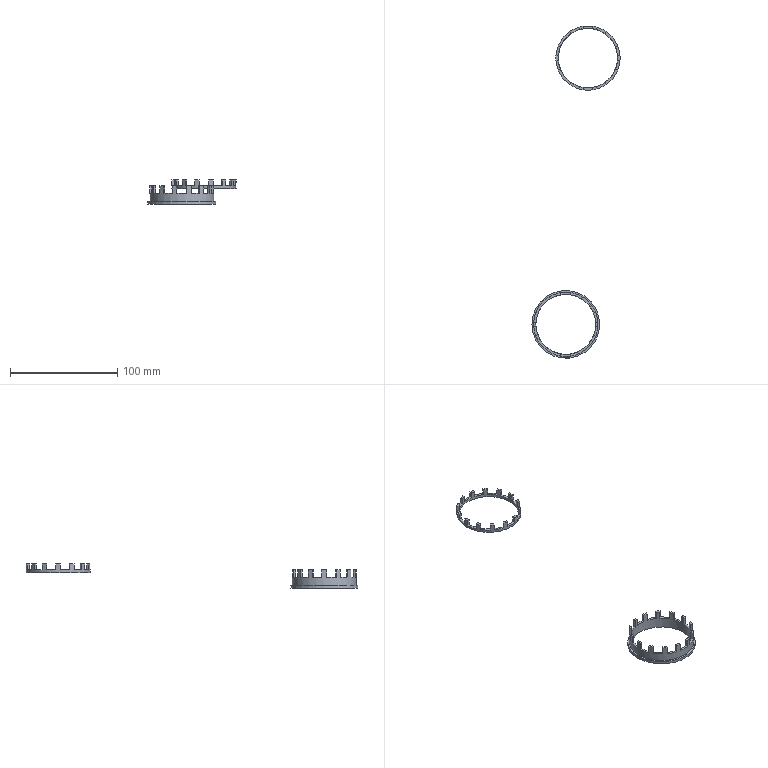NC program | NX | posted with a generic post | part box 82.344 x 310.506 x 22.5 mm
Lines 1 to 1001 of 7127:
N10 G17 G21 G94 G90
(ZLEVEL_PROFILE_COPY_13 , TOOL : D6)
N12 T06 M6
N14 G54
N16 G17 G0 G90 X-0.851 Y-23.489 S9500 M3
N18 G43 Z38. H6
N20 Z7.711
N22 G41 G94 G1 X-0.945 Y-23.523 F1000. D6
N24 X-1.203 Y-23.672
N26 G3 X-1.503 Y-24.192 R0.6
N28 G1 X-1.5 Y-27.4 F2200.
N30 Y-29.387
N32 Y-32.959
N34 G3 X-1.2 Y-33.479 R0.6
N36 G1 X-0.961 Y-33.617
N38 G40
N40 X-0.867 Y-33.651
N42 X0.891 Y-33.745
N44 G41 X0.984 Y-33.707 F1000.
N46 X1.226 Y-33.555
N48 G3 X1.506 Y-33.024 R0.6
N50 G1 X1.5 Y-32.851 F2200.
N52 Y-29.387
N54 Y-27.383
N56 X1.52 Y-27.041
N58 X1.5 Y-27.028
N60 X1.503 Y-24.192
N62 G3 X1.204 Y-23.672 R0.6
N64 G1 X0.945 Y-23.523
N66 G40
N68 X0.851 Y-23.488
N70 G0 X-0.851 Y-23.489 Z7.421
N72 G41 G1 X-0.945 Y-23.523 F1000.
N74 X-1.203 Y-23.672
N76 G3 X-1.503 Y-24.192 R0.6
N78 G1 X-1.5 Y-27.4 F2200.
N80 Y-29.387
N82 Y-32.959
N84 G3 X-1.2 Y-33.479 R0.6
N86 G1 X-0.961 Y-33.617
N88 G40
N90 X-0.867 Y-33.651
N92 X0.891 Y-33.745
N94 G41 X0.984 Y-33.707 F1000.
N96 X1.226 Y-33.555
N98 G3 X1.506 Y-33.024 R0.6
N100 G1 X1.5 Y-32.851 F2200.
N102 Y-29.387
N104 Y-27.383
N106 X1.52 Y-27.041
N108 X1.5 Y-27.028
N110 X1.503 Y-24.192
N112 G3 X1.204 Y-23.672 R0.6
N114 G1 X0.945 Y-23.523
N116 G40
N118 X0.851 Y-23.488
N120 G0 X-0.85 Y-23.489 Z7.132
N122 G41 G1 X-0.944 Y-23.523 F1000.
N124 X-1.203 Y-23.673
N126 G3 X-1.503 Y-24.192 R0.6
N128 G1 X-1.5 Y-27.4 F2200.
N130 Y-29.387
N132 Y-32.959
N134 G3 X-1.2 Y-33.479 R0.6
N136 G1 X-0.961 Y-33.617
N138 G40
N140 X-0.867 Y-33.651
N142 X0.891 Y-33.745
N144 G41 X0.984 Y-33.707 F1000.
N146 X1.226 Y-33.555
N148 G3 X1.506 Y-33.024 R0.6
N150 G1 X1.5 Y-32.851 F2200.
N152 Y-29.387
N154 Y-27.383
N156 X1.52 Y-27.041
N158 X1.5 Y-27.028
N160 X1.503 Y-24.192
N162 G3 X1.204 Y-23.672 R0.6
N164 G1 X0.945 Y-23.523
N166 G40
N168 X0.851 Y-23.488
N170 G0 X-0.85 Y-23.489 Z6.842
N172 G41 G1 X-0.944 Y-23.523 F1000.
N174 X-1.203 Y-23.673
N176 G3 X-1.503 Y-24.192 R0.6
N178 G1 X-1.5 Y-27.4 F2200.
N180 Y-29.387
N182 Y-32.959
N184 G3 X-1.2 Y-33.479 R0.6
N186 G1 X-0.96 Y-33.617
N188 G40
N190 X-0.866 Y-33.651
N192 X0.891 Y-33.745
N194 G41 X0.984 Y-33.707 F1000.
N196 X1.226 Y-33.555
N198 G3 X1.506 Y-33.024 R0.6
N200 G1 X1.5 Y-32.851 F2200.
N202 Y-29.387
N204 Y-27.383
N206 X1.52 Y-27.041
N208 X1.5 Y-27.028
N210 X1.503 Y-24.192
N212 G3 X1.204 Y-23.672 R0.6
N214 G1 X0.945 Y-23.523
N216 G40
N218 X0.851 Y-23.488
N220 G0 X-0.85 Y-23.489 Z6.553
N222 G41 G1 X-0.944 Y-23.523 F1000.
N224 X-1.203 Y-23.673
N226 G3 X-1.502 Y-24.192 R0.6
N228 G1 X-1.5 Y-27.4 F2200.
N230 Y-29.387
N232 Y-32.959
N234 G3 X-1.199 Y-33.479 R0.6
N236 G1 X-0.96 Y-33.617
N238 G40
N240 X-0.866 Y-33.651
N242 X0.891 Y-33.745
N244 G41 X0.984 Y-33.707 F1000.
N246 X1.226 Y-33.555
N248 G3 X1.506 Y-33.024 R0.6
N250 G1 X1.5 Y-32.851 F2200.
N252 Y-29.387
N254 Y-27.383
N256 X1.52 Y-27.041
N258 X1.5 Y-27.028
N260 X1.503 Y-24.192
N262 G3 X1.204 Y-23.672 R0.6
N264 G1 X0.945 Y-23.523
N266 G40
N268 X0.851 Y-23.488
N270 G0 X-0.85 Y-23.489 Z6.263
N272 G41 G1 X-0.944 Y-23.523 F1000.
N274 X-1.203 Y-23.673
N276 G3 X-1.502 Y-24.192 R0.6
N278 G1 X-1.5 Y-27.4 F2200.
N280 Y-29.387
N282 X-1.499 Y-32.959
N284 G3 X-1.199 Y-33.479 R0.6
N286 G1 X-0.96 Y-33.617
N288 G40
N290 X-0.866 Y-33.651
N292 X0.891 Y-33.745
N294 G41 X0.984 Y-33.707 F1000.
N296 X1.226 Y-33.555
N298 G3 X1.506 Y-33.024 R0.6
N300 G1 X1.499 Y-32.851 F2200.
N302 X1.5 Y-29.387
N304 X1.499 Y-27.383
N306 X1.52 Y-27.041
N308 X1.499 Y-27.028
N310 X1.503 Y-24.192
N312 G3 X1.204 Y-23.672 R0.6
N314 G1 X0.945 Y-23.523
N316 G40
N318 X0.851 Y-23.488
N320 G0 X-0.85 Y-23.489 Z5.974
N322 G41 G1 X-0.944 Y-23.523 F1000.
N324 X-1.203 Y-23.673
N326 G3 X-1.502 Y-24.192 R0.6
N328 G1 X-1.5 Y-27.4 F2200.
N330 Y-29.387
N332 X-1.499 Y-32.959
N334 G3 X-1.199 Y-33.479 R0.6
N336 G1 X-0.96 Y-33.617
N338 G40
N340 X-0.866 Y-33.651
N342 X0.891 Y-33.745
N344 G41 X0.984 Y-33.707 F1000.
N346 X1.226 Y-33.555
N348 G3 X1.506 Y-33.024 R0.6
N350 G1 X1.499 Y-32.851 F2200.
N352 X1.5 Y-29.387
N354 X1.499 Y-27.383
N356 X1.52 Y-27.041
N358 X1.499 Y-27.028
N360 X1.503 Y-24.192
N362 G3 X1.204 Y-23.672 R0.6
N364 G1 X0.945 Y-23.523
N366 G40
N368 X0.851 Y-23.488
N370 G0 X-0.85 Y-23.489 Z5.684
N372 G41 G1 X-0.944 Y-23.523 F1000.
N374 X-1.203 Y-23.673
N376 G3 X-1.502 Y-24.192 R0.6
N378 G1 X-1.5 Y-27.4 F2200.
N380 Y-29.387
N382 X-1.499 Y-32.959
N384 G3 X-1.199 Y-33.479 R0.6
N386 G1 X-0.96 Y-33.617
N388 G40
N390 X-0.866 Y-33.651
N392 X0.891 Y-33.745
N394 G41 X0.983 Y-33.707 F1000.
N396 X1.226 Y-33.555
N398 G3 X1.506 Y-33.024 R0.6
N400 G1 X1.499 Y-32.851 F2200.
N402 X1.5 Y-29.387
N404 X1.499 Y-27.383
N406 X1.52 Y-27.041
N408 X1.499 Y-27.028
N410 X1.503 Y-24.192
N412 G3 X1.204 Y-23.672 R0.6
N414 G1 X0.945 Y-23.523
N416 G40
N418 X0.851 Y-23.488
N420 G0 X-0.85 Y-23.489 Z5.395
N422 G41 G1 X-0.944 Y-23.523 F1000.
N424 X-1.202 Y-23.673
N426 G3 X-1.502 Y-24.192 R0.6
N428 G1 X-1.5 Y-27.4 F2200.
N430 Y-29.387
N432 X-1.499 Y-32.959
N434 G3 X-1.199 Y-33.479 R0.6
N436 G1 X-0.96 Y-33.617
N438 G40
N440 X-0.866 Y-33.651
N442 X0.891 Y-33.745
N444 G41 X0.983 Y-33.707 F1000.
N446 X1.226 Y-33.555
N448 G3 X1.506 Y-33.024 R0.6
N450 G1 X1.499 Y-32.851 F2200.
N452 X1.5 Y-29.387
N454 X1.499 Y-27.383
N456 X1.52 Y-27.041
N458 X1.499 Y-27.028
N460 X1.503 Y-24.192
N462 G3 X1.204 Y-23.672 R0.6
N464 G1 X0.945 Y-23.522
N466 G40
N468 X0.851 Y-23.488
N470 G0 X-0.85 Y-23.489 Z5.105
N472 G41 G1 X-0.944 Y-23.523 F1000.
N474 X-1.202 Y-23.673
N476 G3 X-1.502 Y-24.192 R0.6
N478 G1 X-1.5 Y-27.4 F2200.
N480 Y-29.387
N482 X-1.499 Y-32.959
N484 G3 X-1.199 Y-33.479 R0.6
N486 G1 X-0.96 Y-33.617
N488 G40
N490 X-0.866 Y-33.651
N492 X0.891 Y-33.745
N494 G41 X0.983 Y-33.707 F1000.
N496 X1.226 Y-33.555
N498 G3 X1.506 Y-33.024 R0.6
N500 G1 X1.499 Y-32.851 F2200.
N502 X1.5 Y-29.387
N504 X1.499 Y-27.383
N506 X1.52 Y-27.041
N508 X1.499 Y-27.028
N510 X1.503 Y-24.192
N512 G3 X1.204 Y-23.672 R0.6
N514 G1 X0.945 Y-23.522
N516 G40
N518 X0.851 Y-23.488
N520 G0 X-0.85 Y-23.489 Z4.816
N522 G41 G1 X-0.944 Y-23.523 F1000.
N524 X-1.202 Y-23.673
N526 G3 X-1.502 Y-24.192 R0.6
N528 G1 X-1.5 Y-27.4 F2200.
N530 Y-29.387
N532 X-1.499 Y-32.959
N534 G3 X-1.199 Y-33.479 R0.6
N536 G1 X-0.96 Y-33.617
N538 G40
N540 X-0.866 Y-33.651
N542 X0.891 Y-33.745
N544 G41 X0.983 Y-33.707 F1000.
N546 X1.226 Y-33.555
N548 G3 X1.506 Y-33.024 R0.6
N550 G1 X1.499 Y-32.851 F2200.
N552 X1.5 Y-29.387
N554 X1.499 Y-27.383
N556 X1.52 Y-27.041
N558 X1.499 Y-27.028
N560 X1.503 Y-24.192
N562 G3 X1.204 Y-23.672 R0.6
N564 G1 X0.945 Y-23.522
N566 G40
N568 X0.851 Y-23.488
N570 G0 X-0.85 Y-23.489 Z4.526
N572 G41 G1 X-0.944 Y-23.523 F1000.
N574 X-1.202 Y-23.673
N576 G3 X-1.502 Y-24.192 R0.6
N578 G1 X-1.5 Y-27.4 F2200.
N580 Y-29.387
N582 X-1.499 Y-32.959
N584 G3 X-1.199 Y-33.479 R0.6
N586 G1 X-0.96 Y-33.617
N588 G40
N590 X-0.866 Y-33.651
N592 X0.891 Y-33.745
N594 G41 X0.983 Y-33.708 F1000.
N596 X1.226 Y-33.555
N598 G3 X1.506 Y-33.024 R0.6
N600 G1 X1.499 Y-32.851 F2200.
N602 X1.5 Y-29.387
N604 X1.499 Y-27.383
N606 X1.52 Y-27.041
N608 X1.499 Y-27.028
N610 X1.503 Y-24.192
N612 G3 X1.204 Y-23.672 R0.6
N614 G1 X0.945 Y-23.522
N616 G40
N618 X0.851 Y-23.488
N620 G0 X-0.85 Y-23.489 Z4.237
N622 G41 G1 X-0.944 Y-23.523 F1000.
N624 X-1.202 Y-23.673
N626 G3 X-1.502 Y-24.192 R0.6
N628 G1 X-1.5 Y-27.4 F2200.
N630 Y-29.387
N632 X-1.499 Y-32.959
N634 G3 X-1.199 Y-33.479 R0.6
N636 G1 X-0.96 Y-33.617
N638 G40
N640 X-0.866 Y-33.651
N642 X0.891 Y-33.745
N644 G41 X0.983 Y-33.708 F1000.
N646 X1.226 Y-33.555
N648 G3 X1.506 Y-33.024 R0.6
N650 G1 X1.499 Y-32.851 F2200.
N652 X1.5 Y-29.387
N654 X1.499 Y-27.383
N656 X1.52 Y-27.041
N658 X1.499 Y-27.028
N660 X1.503 Y-24.192
N662 G3 X1.204 Y-23.672 R0.6
N664 G1 X0.945 Y-23.522
N666 G40
N668 X0.851 Y-23.488
N670 G0 X-0.849 Y-23.489 Z3.947
N672 G41 G1 X-0.943 Y-23.523 F1000.
N674 X-1.202 Y-23.673
N676 G3 X-1.502 Y-24.192 R0.6
N678 G1 X-1.5 Y-27.4 F2200.
N680 Y-29.387
N682 X-1.499 Y-32.959
N684 G3 X-1.199 Y-33.479 R0.6
N686 G1 X-0.96 Y-33.617
N688 G40
N690 X-0.866 Y-33.651
N692 X0.891 Y-33.745
N694 G41 X0.983 Y-33.708 F1000.
N696 X1.226 Y-33.555
N698 G3 X1.506 Y-33.024 R0.6
N700 G1 X1.499 Y-32.851 F2200.
N702 X1.5 Y-29.387
N704 Y-27.4
N706 X1.499 Y-27.383
N708 X1.52 Y-27.041
N710 X1.499 Y-27.028
N712 X1.503 Y-24.192
N714 G3 X1.204 Y-23.672 R0.6
N716 G1 X0.945 Y-23.522
N718 G40
N720 X0.851 Y-23.488
N722 G0 X-0.849 Y-23.489 Z3.658
N724 G41 G1 X-0.943 Y-23.523 F1000.
N726 X-1.202 Y-23.673
N728 G3 X-1.502 Y-24.192 R0.6
N730 G1 X-1.5 Y-27.4 F2200.
N732 Y-29.387
N734 X-1.499 Y-32.959
N736 G3 X-1.199 Y-33.479 R0.6
N738 G1 X-0.96 Y-33.617
N740 G40
N742 X-0.866 Y-33.651
N744 X0.891 Y-33.745
N746 G41 X0.983 Y-33.708 F1000.
N748 X1.226 Y-33.555
N750 G3 X1.506 Y-33.024 R0.6
N752 G1 X1.499 Y-32.851 F2200.
N754 X1.5 Y-29.387
N756 Y-27.4
N758 X1.499 Y-27.383
N760 X1.518 Y-27.052
N762 X1.502 Y-27.057
N764 X1.491 Y-27.043
N766 X1.499 Y-27.028
N768 X1.503 Y-24.192
N770 G3 X1.204 Y-23.672 R0.6
N772 G1 X0.945 Y-23.522
N774 G40
N776 X0.851 Y-23.488
N778 G0 X-0.849 Y-23.489 Z3.368
N780 G41 G1 X-0.943 Y-23.523 F1000.
N782 X-1.202 Y-23.673
N784 G3 X-1.501 Y-24.192 R0.6
N786 G1 X-1.5 Y-27.4 F2200.
N788 Y-29.387
N790 X-1.499 Y-32.959
N792 G3 X-1.199 Y-33.479 R0.6
N794 G1 X-0.96 Y-33.617
N796 G40
N798 X-0.866 Y-33.651
N800 X0.891 Y-33.746
N802 G41 X0.983 Y-33.708 F1000.
N804 X1.226 Y-33.555
N806 G3 X1.505 Y-33.024 R0.6
N808 G1 X1.499 Y-32.851 F2200.
N810 X1.5 Y-29.387
N812 Y-27.4
N814 X1.499 Y-27.383
N816 X1.518 Y-27.052
N818 X1.502 Y-27.057
N820 X1.491 Y-27.043
N822 X1.499 Y-27.028
N824 X1.503 Y-24.192
N826 G3 X1.204 Y-23.672 R0.6
N828 G1 X0.945 Y-23.522
N830 G40
N832 X0.851 Y-23.488
N834 G0 X-0.849 Y-23.489 Z3.079
N836 G41 G1 X-0.943 Y-23.523 F1000.
N838 X-1.202 Y-23.673
N840 G3 X-1.501 Y-24.192 R0.6
N842 G1 X-1.5 Y-27.4 F2200.
N844 Y-29.387
N846 X-1.499 Y-32.959
N848 G3 X-1.199 Y-33.479 R0.6
N850 G1 X-0.96 Y-33.617
N852 G40
N854 X-0.866 Y-33.651
N856 X0.891 Y-33.746
N858 G41 X0.983 Y-33.708 F1000.
N860 X1.226 Y-33.555
N862 G3 X1.505 Y-33.024 R0.6
N864 G1 X1.499 Y-32.851 F2200.
N866 X1.5 Y-29.387
N868 Y-27.4
N870 X1.499 Y-27.383
N872 X1.518 Y-27.052
N874 X1.502 Y-27.057
N876 X1.491 Y-27.043
N878 X1.499 Y-27.028
N880 X1.503 Y-24.192
N882 G3 X1.203 Y-23.672 R0.6
N884 G1 X0.945 Y-23.522
N886 G40
N888 X0.851 Y-23.488
N890 G0 X-0.849 Y-23.489 Z2.789
N892 G41 G1 X-0.943 Y-23.523 F1000.
N894 X-1.202 Y-23.673
N896 G3 X-1.501 Y-24.192 R0.6
N898 G1 X-1.5 Y-27.4 F2200.
N900 Y-29.387
N902 X-1.499 Y-32.959
N904 G3 X-1.198 Y-33.479 R0.6
N906 G1 X-0.96 Y-33.617
N908 G40
N910 X-0.866 Y-33.651
N912 X0.89 Y-33.746
N914 G41 X0.983 Y-33.708 F1000.
N916 X1.226 Y-33.555
N918 G3 X1.505 Y-33.024 R0.6
N920 G1 X1.499 Y-32.851 F2200.
N922 X1.5 Y-29.387
N924 Y-27.4
N926 X1.499 Y-27.383
N928 X1.518 Y-27.052
N930 X1.499 Y-27.039
N932 X1.503 Y-24.192
N934 G3 X1.203 Y-23.672 R0.6
N936 G1 X0.945 Y-23.522
N938 G40
N940 X0.851 Y-23.488
N942 G0 X-0.849 Y-23.489 Z2.5
N944 G41 G1 X-0.943 Y-23.523 F1000.
N946 X-1.201 Y-23.673
N948 G3 X-1.501 Y-24.192 R0.6
N950 G1 X-1.5 Y-27.4 F2200.
N952 Y-29.387
N954 X-1.499 Y-32.959
N956 G3 X-1.198 Y-33.479 R0.6
N958 G1 X-0.959 Y-33.617
N960 G40
N962 X-0.865 Y-33.651
N964 X0.89 Y-33.746
N966 G41 X0.983 Y-33.708 F1000.
N968 X1.226 Y-33.555
N970 G3 X1.505 Y-33.024 R0.6
N972 G1 X1.499 Y-32.851 F2200.
N974 X1.5 Y-29.387
N976 Y-27.4
N978 X1.499 Y-27.383
N980 X1.518 Y-27.052
N982 X1.499 Y-27.039
N984 X1.503 Y-24.192
N986 G3 X1.203 Y-23.672 R0.6
N988 G1 X0.945 Y-23.522
N990 G40
N992 X0.851 Y-23.488
N994 G0 Z38.
(ZLEVEL_PROFILE_COPY_13_COPY , TOOL : D6)
N996 X9.425 Y-21.532
N998 Z7.711
N1000 G41 G1 X9.355 Y-21.603 F1000.
N1002 X9.187 Y-21.85
N1004 G3 X9.143 Y-22.449 R0.6
N1006 G1 X10.537 Y-25.337 F2200.
N1008 X11.399 Y-27.128
N1010 X12.949 Y-30.346
N1012 G3 X13.445 Y-30.684 R0.6
N1014 G1 X13.72 Y-30.705
N1016 G40
N1018 X13.82 Y-30.695
N1020 X15.444 Y-30.016
N1022 G41 X15.511 Y-29.942 F1000.
N1024 X15.663 Y-29.7
N1026 G3 X15.686 Y-29.1 R0.6
N1028 G1 X15.605 Y-28.947 F2200.
N1030 X14.102 Y-25.826
N1032 X13.232 Y-24.02
N1034 X13.102 Y-23.704
N1036 X13.078 Y-23.701
N1038 X11.851 Y-21.144
N1040 G3 X11.356 Y-20.806 R0.6
N1042 G1 X11.058 Y-20.783
N1044 G40
N1046 X10.958 Y-20.793
N1048 G0 X9.425 Y-21.532 Z7.421
N1050 G41 G1 X9.355 Y-21.603 F1000.
N1052 X9.187 Y-21.85
N1054 G3 X9.143 Y-22.449 R0.6
N1056 G1 X10.537 Y-25.337 F2200.
N1058 X11.399 Y-27.128
N1060 X12.949 Y-30.346
N1062 G3 X13.445 Y-30.684 R0.6
N1064 G1 X13.72 Y-30.704
N1066 G40
N1068 X13.82 Y-30.695
N1070 X15.444 Y-30.016
N1072 G41 X15.511 Y-29.942 F1000.
N1074 X15.663 Y-29.7
N1076 G3 X15.686 Y-29.1 R0.6
N1078 G1 X15.605 Y-28.947 F2200.
N1080 X14.102 Y-25.826
N1082 X13.232 Y-24.02
N1084 X13.102 Y-23.704
N1086 X13.078 Y-23.701
N1088 X11.851 Y-21.144
N1090 G3 X11.356 Y-20.806 R0.6
N1092 G1 X11.058 Y-20.783
N1094 G40
N1096 X10.958 Y-20.793
N1098 G0 X9.425 Y-21.532 Z7.132
N1100 G41 G1 X9.355 Y-21.603 F1000.
N1102 X9.187 Y-21.85
N1104 G3 X9.143 Y-22.449 R0.6
N1106 G1 X10.537 Y-25.337 F2200.
N1108 X11.399 Y-27.128
N1110 X12.949 Y-30.346
N1112 G3 X13.445 Y-30.684 R0.6
N1114 G1 X13.72 Y-30.704
N1116 G40
N1118 X13.82 Y-30.694
N1120 X15.444 Y-30.016
N1122 G41 X15.511 Y-29.942 F1000.
N1124 X15.663 Y-29.7
N1126 G3 X15.686 Y-29.1 R0.6
N1128 G1 X15.605 Y-28.947 F2200.
N1130 X14.102 Y-25.826
N1132 X13.232 Y-24.02
N1134 X13.102 Y-23.704
N1136 X13.078 Y-23.701
N1138 X11.851 Y-21.144
N1140 G3 X11.356 Y-20.806 R0.6
N1142 G1 X11.058 Y-20.783
N1144 G40
N1146 X10.958 Y-20.793
N1148 G0 X9.425 Y-21.532 Z6.842
N1150 G41 G1 X9.355 Y-21.603 F1000.
N1152 X9.187 Y-21.85
N1154 G3 X9.143 Y-22.449 R0.6
N1156 G1 X10.537 Y-25.337 F2200.
N1158 X11.399 Y-27.128
N1160 X12.949 Y-30.346
N1162 G3 X13.445 Y-30.684 R0.6
N1164 G1 X13.72 Y-30.704
N1166 G40
N1168 X13.82 Y-30.694
N1170 X15.444 Y-30.016
N1172 G41 X15.511 Y-29.942 F1000.
N1174 X15.663 Y-29.7
N1176 G3 X15.686 Y-29.1 R0.6
N1178 G1 X15.605 Y-28.947 F2200.
N1180 X14.102 Y-25.826
N1182 X13.232 Y-24.02
N1184 X13.102 Y-23.704
N1186 X13.078 Y-23.701
N1188 X11.851 Y-21.144
N1190 G3 X11.356 Y-20.806 R0.6
N1192 G1 X11.058 Y-20.783
N1194 G40
N1196 X10.958 Y-20.793
N1198 G0 X9.425 Y-21.531 Z6.553
N1200 G41 G1 X9.355 Y-21.603 F1000.
N1202 X9.187 Y-21.85
N1204 G3 X9.143 Y-22.448 R0.6
N1206 G1 X10.537 Y-25.337 F2200.
N1208 X11.399 Y-27.128
N1210 X12.949 Y-30.346
N1212 G3 X13.445 Y-30.684 R0.6
N1214 G1 X13.72 Y-30.704
N1216 G40
N1218 X13.82 Y-30.694
N1220 X15.444 Y-30.016
N1222 G41 X15.511 Y-29.942 F1000.
N1224 X15.663 Y-29.7
N1226 G3 X15.686 Y-29.1 R0.6
N1228 G1 X15.604 Y-28.947 F2200.
N1230 X14.102 Y-25.826
N1232 X13.232 Y-24.02
N1234 X13.102 Y-23.704
N1236 X13.078 Y-23.701
N1238 X11.851 Y-21.144
N1240 G3 X11.356 Y-20.806 R0.6
N1242 G1 X11.058 Y-20.783
N1244 G40
N1246 X10.958 Y-20.793
N1248 G0 X9.425 Y-21.531 Z6.263
N1250 G41 G1 X9.356 Y-21.603 F1000.
N1252 X9.187 Y-21.85
N1254 G3 X9.143 Y-22.448 R0.6
N1256 G1 X10.537 Y-25.337 F2200.
N1258 X11.399 Y-27.128
N1260 X12.949 Y-30.346
N1262 G3 X13.445 Y-30.684 R0.6
N1264 G1 X13.721 Y-30.704
N1266 G40
N1268 X13.82 Y-30.694
N1270 X15.444 Y-30.017
N1272 G41 X15.511 Y-29.942 F1000.
N1274 X15.663 Y-29.7
N1276 G3 X15.685 Y-29.1 R0.6
N1278 G1 X15.604 Y-28.947 F2200.
N1280 X14.102 Y-25.826
N1282 X13.232 Y-24.02
N1284 X13.102 Y-23.704
N1286 X13.078 Y-23.701
N1288 X11.851 Y-21.144
N1290 G3 X11.356 Y-20.806 R0.6
N1292 G1 X11.058 Y-20.783
N1294 G40
N1296 X10.958 Y-20.793
N1298 G0 X9.425 Y-21.531 Z5.974
N1300 G41 G1 X9.356 Y-21.603 F1000.
N1302 X9.188 Y-21.85
N1304 G3 X9.143 Y-22.448 R0.6
N1306 G1 X10.537 Y-25.337 F2200.
N1308 X11.399 Y-27.128
N1310 X12.95 Y-30.346
N1312 G3 X13.445 Y-30.684 R0.6
N1314 G1 X13.721 Y-30.704
N1316 G40
N1318 X13.82 Y-30.694
N1320 X15.444 Y-30.017
N1322 G41 X15.511 Y-29.942 F1000.
N1324 X15.663 Y-29.7
N1326 G3 X15.685 Y-29.1 R0.6
N1328 G1 X15.604 Y-28.947 F2200.
N1330 X14.102 Y-25.826
N1332 X13.232 Y-24.02
N1334 X13.102 Y-23.704
N1336 X13.078 Y-23.701
N1338 X11.851 Y-21.144
N1340 G3 X11.356 Y-20.806 R0.6
N1342 G1 X11.058 Y-20.783
N1344 G40
N1346 X10.958 Y-20.793
N1348 G0 X9.426 Y-21.531 Z5.684
N1350 G41 G1 X9.356 Y-21.603 F1000.
N1352 X9.188 Y-21.85
N1354 G3 X9.143 Y-22.448 R0.6
N1356 G1 X10.537 Y-25.337 F2200.
N1358 X11.399 Y-27.128
N1360 X12.95 Y-30.346
N1362 G3 X13.445 Y-30.684 R0.6
N1364 G1 X13.721 Y-30.704
N1366 G40
N1368 X13.82 Y-30.694
N1370 X15.444 Y-30.017
N1372 G41 X15.511 Y-29.943 F1000.
N1374 X15.663 Y-29.7
N1376 G3 X15.685 Y-29.1 R0.6
N1378 G1 X15.604 Y-28.947 F2200.
N1380 X14.102 Y-25.826
N1382 X13.232 Y-24.02
N1384 X13.102 Y-23.704
N1386 X13.078 Y-23.701
N1388 X11.851 Y-21.144
N1390 G3 X11.356 Y-20.806 R0.6
N1392 G1 X11.058 Y-20.783
N1394 G40
N1396 X10.958 Y-20.793
N1398 G0 X9.426 Y-21.531 Z5.395
N1400 G41 G1 X9.356 Y-21.603 F1000.
N1402 X9.188 Y-21.85
N1404 G3 X9.143 Y-22.448 R0.6
N1406 G1 X10.537 Y-25.337 F2200.
N1408 X11.399 Y-27.128
N1410 X12.95 Y-30.346
N1412 G3 X13.445 Y-30.684 R0.6
N1414 G1 X13.721 Y-30.704
N1416 G40
N1418 X13.82 Y-30.694
N1420 X15.444 Y-30.017
N1422 G41 X15.511 Y-29.943 F1000.
N1424 X15.663 Y-29.7
N1426 G3 X15.685 Y-29.1 R0.6
N1428 G1 X15.604 Y-28.947 F2200.
N1430 X14.102 Y-25.826
N1432 X13.232 Y-24.02
N1434 X13.102 Y-23.704
N1436 X13.078 Y-23.701
N1438 X11.851 Y-21.144
N1440 G3 X11.356 Y-20.806 R0.6
N1442 G1 X11.057 Y-20.783
N1444 G40
N1446 X10.958 Y-20.793
N1448 G0 X9.426 Y-21.531 Z5.105
N1450 G41 G1 X9.356 Y-21.603 F1000.
N1452 X9.188 Y-21.85
N1454 G3 X9.143 Y-22.448 R0.6
N1456 G1 X10.537 Y-25.337 F2200.
N1458 X11.399 Y-27.128
N1460 X12.95 Y-30.346
N1462 G3 X13.446 Y-30.684 R0.6
N1464 G1 X13.721 Y-30.704
N1466 G40
N1468 X13.82 Y-30.694
N1470 X15.444 Y-30.017
N1472 G41 X15.511 Y-29.943 F1000.
N1474 X15.663 Y-29.7
N1476 G3 X15.685 Y-29.1 R0.6
N1478 G1 X15.604 Y-28.947 F2200.
N1480 X14.102 Y-25.826
N1482 X13.232 Y-24.02
N1484 X13.102 Y-23.704
N1486 X13.078 Y-23.701
N1488 X11.851 Y-21.144
N1490 G3 X11.356 Y-20.806 R0.6
N1492 G1 X11.057 Y-20.783
N1494 G40
N1496 X10.958 Y-20.793
N1498 G0 X9.426 Y-21.531 Z4.816
N1500 G41 G1 X9.356 Y-21.603 F1000.
N1502 X9.188 Y-21.85
N1504 G3 X9.143 Y-22.448 R0.6
N1506 G1 X10.537 Y-25.337 F2200.
N1508 X11.399 Y-27.128
N1510 X12.95 Y-30.346
N1512 G3 X13.446 Y-30.684 R0.6
N1514 G1 X13.721 Y-30.704
N1516 G40
N1518 X13.82 Y-30.694
N1520 X15.444 Y-30.017
N1522 G41 X15.511 Y-29.943 F1000.
N1524 X15.663 Y-29.7
N1526 G3 X15.685 Y-29.1 R0.6
N1528 G1 X15.604 Y-28.947 F2200.
N1530 X14.102 Y-25.826
N1532 X13.232 Y-24.021
N1534 X13.102 Y-23.704
N1536 X13.078 Y-23.701
N1538 X11.851 Y-21.144
N1540 G3 X11.356 Y-20.806 R0.6
N1542 G1 X11.057 Y-20.783
N1544 G40
N1546 X10.958 Y-20.793
N1548 G0 X9.426 Y-21.531 Z4.526
N1550 G41 G1 X9.356 Y-21.603 F1000.
N1552 X9.188 Y-21.85
N1554 G3 X9.144 Y-22.448 R0.6
N1556 G1 X10.537 Y-25.337 F2200.
N1558 X11.399 Y-27.128
N1560 X12.95 Y-30.346
N1562 G3 X13.446 Y-30.684 R0.6
N1564 G1 X13.721 Y-30.704
N1566 G40
N1568 X13.82 Y-30.694
N1570 X15.444 Y-30.017
N1572 G41 X15.511 Y-29.943 F1000.
N1574 X15.663 Y-29.7
N1576 G3 X15.685 Y-29.1 R0.6
N1578 G1 X15.604 Y-28.947 F2200.
N1580 X14.102 Y-25.826
N1582 X13.232 Y-24.021
N1584 X13.102 Y-23.704
N1586 X13.078 Y-23.701
N1588 X11.851 Y-21.144
N1590 G3 X11.356 Y-20.806 R0.6
N1592 G1 X11.057 Y-20.783
N1594 G40
N1596 X10.958 Y-20.793
N1598 G0 X9.426 Y-21.531 Z4.237
N1600 G41 G1 X9.356 Y-21.603 F1000.
N1602 X9.188 Y-21.85
N1604 G3 X9.144 Y-22.448 R0.6
N1606 G1 X10.537 Y-25.337 F2200.
N1608 X11.399 Y-27.128
N1610 X12.95 Y-30.346
N1612 G3 X13.446 Y-30.683 R0.6
N1614 G1 X13.721 Y-30.704
N1616 G40
N1618 X13.82 Y-30.694
N1620 X15.444 Y-30.017
N1622 G41 X15.511 Y-29.943 F1000.
N1624 X15.663 Y-29.7
N1626 G3 X15.685 Y-29.1 R0.6
N1628 G1 X15.604 Y-28.947 F2200.
N1630 X14.102 Y-25.826
N1632 X13.231 Y-24.021
N1634 X13.102 Y-23.704
N1636 X13.078 Y-23.701
N1638 X11.851 Y-21.144
N1640 G3 X11.355 Y-20.806 R0.6
N1642 G1 X11.057 Y-20.783
N1644 G40
N1646 X10.958 Y-20.793
N1648 G0 X9.426 Y-21.531 Z3.947
N1650 G41 G1 X9.356 Y-21.603 F1000.
N1652 X9.188 Y-21.85
N1654 G3 X9.144 Y-22.448 R0.6
N1656 G1 X10.537 Y-25.337 F2200.
N1658 X11.399 Y-27.128
N1660 X12.95 Y-30.346
N1662 G3 X13.446 Y-30.683 R0.6
N1664 G1 X13.721 Y-30.704
N1666 G40
N1668 X13.821 Y-30.694
N1670 X15.444 Y-30.017
N1672 G41 X15.511 Y-29.943 F1000.
N1674 X15.663 Y-29.7
N1676 G3 X15.685 Y-29.1 R0.6
N1678 G1 X15.604 Y-28.947 F2200.
N1680 X14.102 Y-25.826
N1682 X13.24 Y-24.036
N1684 X13.231 Y-24.021
N1686 X13.102 Y-23.704
N1688 X13.078 Y-23.701
N1690 X11.851 Y-21.145
N1692 G3 X11.355 Y-20.806 R0.6
N1694 G1 X11.057 Y-20.783
N1696 G40
N1698 X10.958 Y-20.793
N1700 G0 X9.426 Y-21.531 Z3.658
N1702 G41 G1 X9.356 Y-21.603 F1000.
N1704 X9.188 Y-21.85
N1706 G3 X9.144 Y-22.448 R0.6
N1708 G1 X10.537 Y-25.337 F2200.
N1710 X11.399 Y-27.128
N1712 X12.95 Y-30.346
N1714 G3 X13.446 Y-30.683 R0.6
N1716 G1 X13.721 Y-30.704
N1718 G40
N1720 X13.821 Y-30.694
N1722 X15.444 Y-30.017
N1724 G41 X15.511 Y-29.943 F1000.
N1726 X15.663 Y-29.7
N1728 G3 X15.685 Y-29.1 R0.6
N1730 G1 X15.604 Y-28.947 F2200.
N1732 X14.102 Y-25.826
N1734 X13.24 Y-24.036
N1736 X13.231 Y-24.021
N1738 X13.105 Y-23.714
N1740 X13.093 Y-23.726
N1742 X13.077 Y-23.718
N1744 Y-23.701
N1746 X11.851 Y-21.145
N1748 G3 X11.355 Y-20.806 R0.6
N1750 G1 X11.057 Y-20.783
N1752 G40
N1754 X10.958 Y-20.793
N1756 G0 X9.426 Y-21.531 Z3.368
N1758 G41 G1 X9.357 Y-21.603 F1000.
N1760 X9.188 Y-21.85
N1762 G3 X9.144 Y-22.448 R0.6
N1764 G1 X10.537 Y-25.337 F2200.
N1766 X11.399 Y-27.128
N1768 X12.95 Y-30.346
N1770 G3 X13.446 Y-30.683 R0.6
N1772 G1 X13.721 Y-30.704
N1774 G40
N1776 X13.821 Y-30.694
N1778 X15.444 Y-30.017
N1780 G41 X15.511 Y-29.943 F1000.
N1782 X15.663 Y-29.7
N1784 G3 X15.685 Y-29.1 R0.6
N1786 G1 X15.604 Y-28.947 F2200.
N1788 X14.102 Y-25.826
N1790 X13.24 Y-24.036
N1792 X13.231 Y-24.021
N1794 X13.105 Y-23.714
N1796 X13.093 Y-23.726
N1798 X13.077 Y-23.718
N1800 Y-23.701
N1802 X11.851 Y-21.145
N1804 G3 X11.355 Y-20.806 R0.6
N1806 G1 X11.057 Y-20.783
N1808 G40
N1810 X10.958 Y-20.793
N1812 G0 X9.426 Y-21.531 Z3.079
N1814 G41 G1 X9.357 Y-21.603 F1000.
N1816 X9.189 Y-21.85
N1818 G3 X9.144 Y-22.448 R0.6
N1820 G1 X10.537 Y-25.337 F2200.
N1822 X11.399 Y-27.128
N1824 X12.95 Y-30.346
N1826 G3 X13.446 Y-30.683 R0.6
N1828 G1 X13.721 Y-30.704
N1830 G40
N1832 X13.821 Y-30.694
N1834 X15.444 Y-30.017
N1836 G41 X15.511 Y-29.943 F1000.
N1838 X15.663 Y-29.7
N1840 G3 X15.685 Y-29.1 R0.6
N1842 G1 X15.604 Y-28.947 F2200.
N1844 X14.102 Y-25.826
N1846 X13.24 Y-24.036
N1848 X13.231 Y-24.021
N1850 X13.105 Y-23.714
N1852 X13.093 Y-23.726
N1854 X13.077 Y-23.718
N1856 Y-23.701
N1858 X11.851 Y-21.145
N1860 G3 X11.355 Y-20.806 R0.6
N1862 G1 X11.057 Y-20.783
N1864 G40
N1866 X10.958 Y-20.793
N1868 G0 X9.426 Y-21.531 Z2.789
N1870 G41 G1 X9.357 Y-21.603 F1000.
N1872 X9.189 Y-21.85
N1874 G3 X9.144 Y-22.448 R0.6
N1876 G1 X10.537 Y-25.337 F2200.
N1878 X11.399 Y-27.128
N1880 X12.95 Y-30.346
N1882 G3 X13.446 Y-30.683 R0.6
N1884 G1 X13.721 Y-30.704
N1886 G40
N1888 X13.821 Y-30.694
N1890 X15.444 Y-30.017
N1892 G41 X15.511 Y-29.943 F1000.
N1894 X15.663 Y-29.7
N1896 G3 X15.685 Y-29.1 R0.6
N1898 G1 X15.604 Y-28.947 F2200.
N1900 X14.102 Y-25.826
N1902 X13.24 Y-24.036
N1904 X13.231 Y-24.021
N1906 X13.105 Y-23.714
N1908 X13.082 Y-23.711
N1910 X11.851 Y-21.145
N1912 G3 X11.355 Y-20.806 R0.6
N1914 G1 X11.057 Y-20.783
N1916 G40
N1918 X10.958 Y-20.793
N1920 G0 X9.427 Y-21.531 Z2.5
N1922 G41 G1 X9.357 Y-21.603 F1000.
N1924 X9.189 Y-21.85
N1926 G3 X9.144 Y-22.448 R0.6
N1928 G1 X10.537 Y-25.337 F2200.
N1930 X11.399 Y-27.128
N1932 X12.95 Y-30.345
N1934 G3 X13.446 Y-30.683 R0.6
N1936 G1 X13.721 Y-30.704
N1938 G40
N1940 X13.821 Y-30.694
N1942 X15.444 Y-30.017
N1944 G41 X15.511 Y-29.943 F1000.
N1946 X15.663 Y-29.7
N1948 G3 X15.685 Y-29.101 R0.6
N1950 G1 X15.604 Y-28.947 F2200.
N1952 X14.102 Y-25.826
N1954 X13.24 Y-24.036
N1956 X13.231 Y-24.021
N1958 X13.105 Y-23.714
N1960 X13.082 Y-23.711
N1962 X11.851 Y-21.145
N1964 G3 X11.355 Y-20.806 R0.6
N1966 G1 X11.057 Y-20.783
N1968 G40
N1970 X10.958 Y-20.793
N1972 G0 Z38.
(ZLEVEL_PROFILE_COPY_13_COPY_1 , TOOL : D6)
N1974 X17.834 Y-15.31
N1976 Z7.711
N1978 G41 G1 X17.802 Y-15.405 F1000.
N1980 X17.758 Y-15.7
N1982 G3 X17.977 Y-16.259 R0.6
N1984 G1 X20.487 Y-18.256 F2200.
N1986 X22.041 Y-19.496
N1988 X24.833 Y-21.722